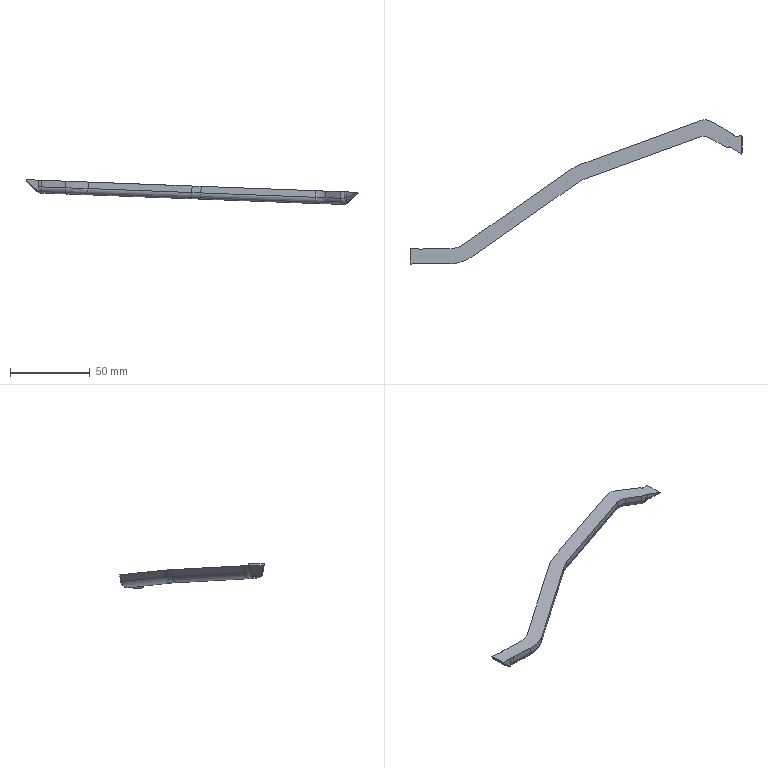Part | Creo | 1 solid | 69 faces | box 207.911 x 90.415 x 15.437 mm | volume 14249 mm3 | spline 22 | plane 21 | cylinder 19 | sphere 6 | torus 1 | commonest cylinder face diameters 8.4 x15 1 x2 16 x2